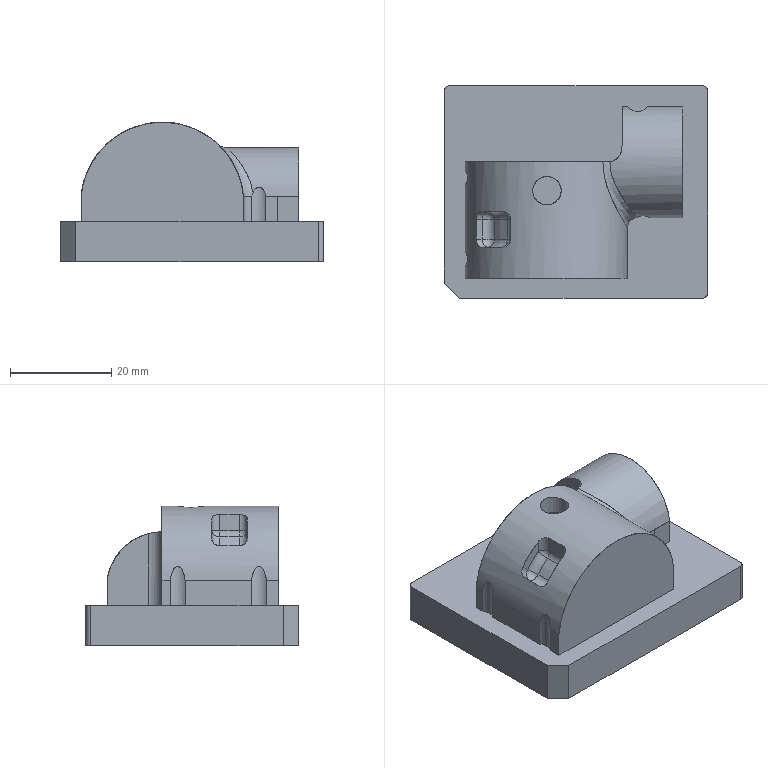NC program | PowerMill | posted with a generic post | part box 52 x 42 x 27.622 mm
Lines 31074 to 31904 of 214543:
N31171 M6
N31172 S18000 M03
N31173 G00 G90 X0.0 Y0.0
N31174 G43 Z9.8022 H28
N31175
N31176 G05 P10000 R4
N31177 X-5.3782 Y0.3338
N31178 Z0.6661
N31179 G01 Z-0.5339 F2400.0
N31180 X-5.0522 Y0.4141 Z-0.5398
N31181 X-4.5942 Z-0.5478
N31182 X-4.1495 Y0.3045 Z-0.5558
N31183 X-3.8382 Y0.1411 Z-0.5619
N31184 X-3.8434 Y0.0036 Z-0.5643
N31185 X-3.9122 Y-0.335 Z-0.5704
N31186 X-4.0514 Y-0.6732 Z-0.5767
N31187 X-4.3199 Y-1.0601 Z-0.585
N31188 X-4.6246 Y-1.3218 Z-0.592
N31189 X-4.8383 Y-1.4461 Z-0.5963
N31190 X-4.9933 Y-1.5363 Z-0.5994
N31191 X-4.997 Y-1.5384 Z-0.5995
N31192 X-5.3352 Y-1.6444 Z-0.6057
N31193 X-5.6736 Y-1.6847 Z-0.6116
N31194 X-6.012 Y-1.6647 Z-0.6175
N31195 X-6.35 Y-1.583 Z-0.6236
N31196 X-6.715 Y-1.4042 Z-0.6307
N31197 X-6.668 Y-1.0173 Z-0.6375
N31198 X-6.5056 Y-0.5891 Z-0.6455
N31199 X-6.2454 Y-0.2121 Z-0.6535
N31200 X-5.9025 Y0.0916 Z-0.6615
N31201 X-5.497 Y0.3045 Z-0.6695
N31202 X-5.0522 Y0.4141 Z-0.6775
N31203 X-4.5942 Z-0.6855
N31204 X-4.1495 Y0.3045 Z-0.6934
N31205 X-3.8382 Y0.1411 Z-0.6996
N31206 X-3.8434 Y0.0036 Z-0.702
N31207 X-3.9122 Y-0.335 Z-0.708
N31208 X-4.0514 Y-0.6732 Z-0.7144
N31209 X-4.3199 Y-1.0601 Z-0.7226
N31210 X-4.6246 Y-1.3218 Z-0.7296
N31211 X-4.8383 Y-1.4461 Z-0.7339
N31212 X-4.8232 Y-1.472
N31213 X-5.305 Y-0.5688 F4000.0
N31214 G03 X-4.8696 Y0.1569 I-0.387 J0.7257
N31215 G03 X-6.5143 I-0.8224 J0.0
N31216 G03 X-5.305 Y-0.5688 I0.8223 J0.0
N31217 G01 X-4.8232 Y-1.472
N31218 X-4.6072 Y-1.3463
N31219 X-4.2975 Y-1.0804
N31220 X-4.0249 Y-0.6876
N31221 X-3.8833 Y-0.3438
N31222 X-3.8136 Y0.0
N31223 X-3.8005 Y0.3438
N31224 X-3.859 Y0.6876
N31225 X-3.9537 Y0.9709
N31226 X-4.1319 Y1.2835
N31227 X-4.284 Y1.4942
N31228 X-4.2975 Y1.5102
N31229 X-4.6413 Y1.8089
N31230 X-4.9851 Y1.9994
N31231 X-5.3289 Y2.1071
N31232 X-5.6727 Y2.1481
N31233 X-6.0165 Y2.1279
N31234 X-6.3004 Y2.0628
N31235 X-6.7041 Y1.8894
N31236 X-6.7094 Y1.8857
N31237 X-6.9842 Y1.6864
N31238 X-7.2966 Y1.3752
N31239 X-7.5019 Y1.0314
N31240 X-7.623 Y0.6876
N31241 X-7.6792 Y0.3438
N31242 X-7.6692 Y0.0
N31243 X-7.5991 Y-0.3438
N31244 X-7.4593 Y-0.6876
N31245 X-7.2269 Y-1.0314
N31246 X-6.8424 Y-1.3752
N31247 X-6.3603 Y-1.6114
N31248 X-6.0165 Y-1.6945
N31249 X-5.6727 Y-1.7148
N31250 X-5.3289 Y-1.6738
N31251 X-4.9851 Y-1.5661
N31252 X-4.9785 Y-1.5624
N31253 X-4.8232 Y-1.472
N31254 X-5.6684 Y0.541 Z-0.6329
N31255 X-5.6503 Y0.6898 Z-0.6355 F2400.0
N31256 X-5.4879 Y1.118 Z-0.6435
N31257 X-5.2277 Y1.495 Z-0.6515
N31258 X-4.8848 Y1.7987 Z-0.6595
N31259 X-4.7821 Y1.8526 Z-0.6615
N31260 X-4.6586 Y1.7842 Z-0.664
N31261 X-4.3189 Y1.4879 Z-0.6719
N31262 X-4.3018 Y1.4676 Z-0.6723
N31263 X-4.1592 Y1.2702 Z-0.6766
N31264 X-3.9812 Y0.957 Z-0.6829
N31265 X-3.8882 Y0.6803 Z-0.688
N31266 X-3.8317 Y0.3418 Z-0.694
N31267 X-3.8355 Y0.2361 Z-0.6958
N31268 X-3.8438 Y0.0035 Z-0.6999
N31269 X-3.9125 Y-0.335 Z-0.7059
N31270 X-4.0522 Y-0.6732 Z-0.7123
N31271 X-4.32 Y-1.06 Z-0.7205
N31272 X-4.6249 Y-1.322 Z-0.7275
N31273 X-4.7541 Y-1.3972 Z-0.7301
N31274 X-4.8848 Y-1.3286 Z-0.7327
N31275 X-5.2277 Y-1.0249 Z-0.7407
N31276 X-5.4879 Y-0.6479 Z-0.7487
N31277 X-5.6503 Y-0.2196 Z-0.7567
N31278 X-5.7055 Y0.2351 Z-0.7647
N31279 X-5.6503 Y0.6898 Z-0.7727
N31280 X-5.4879 Y1.118 Z-0.7807
N31281 X-5.2277 Y1.495 Z-0.7887
N31282 X-4.8848 Y1.7987 Z-0.7966
N31283 X-4.7821 Y1.8526 Z-0.7987
N31284 X-4.6586 Y1.7842 Z-0.8011
N31285 X-4.3189 Y1.4879 Z-0.809
N31286 X-4.3018 Y1.4676 Z-0.8095
N31287 X-4.1592 Y1.2702 Z-0.8137
N31288 X-3.9812 Y0.957 Z-0.82
N31289 X-3.8882 Y0.6803 Z-0.8251
N31290 X-3.8317 Y0.3418 Z-0.8311
N31291 X-3.8355 Y0.2361 Z-0.8329
N31292 X-3.8055 Y0.2351
N31293 X-4.8263 F4000.0
N31294 G03 X-6.4843 I-0.829 J0.0
N31295 G03 X-4.8263 I0.829 J0.0
N31296 G01 X-3.8055
N31297 X-3.8016 Y0.3438
N31298 X-3.859 Y0.6876
N31299 X-3.9537 Y0.9693
N31300 X-4.134 Y1.2865
N31301 X-4.2781 Y1.4861
N31302 X-4.2975 Y1.509
N31303 X-4.6413 Y1.8089
N31304 X-4.9851 Y1.9994
N31305 X-5.3289 Y2.1071
N31306 X-5.6727 Y2.1481
N31307 X-6.0165 Y2.1279
N31308 X-6.3003 Y2.0628
N31309 X-6.7041 Y1.8894
N31310 X-6.7112 Y1.8844
N31311 X-6.9835 Y1.687
N31312 X-7.2953 Y1.3752
N31313 X-7.5006 Y1.0314
N31314 X-7.6218 Y0.6876
N31315 X-7.677 Y0.3438
N31316 X-7.6686 Y0.0
N31317 X-7.5986 Y-0.3438
N31318 X-7.4585 Y-0.6876
N31319 X-7.2258 Y-1.0314
N31320 X-6.8424 Y-1.3752
N31321 X-6.3603 Y-1.6114
N31322 X-6.0165 Y-1.6945
N31323 X-5.6727 Y-1.7148
N31324 X-5.3289 Y-1.6738
N31325 X-4.9851 Y-1.5661
N31326 X-4.9763 Y-1.5612
N31327 X-4.6074 Y-1.3465
N31328 X-4.2975 Y-1.0803
N31329 X-4.0257 Y-0.6876
N31330 X-3.8837 Y-0.3438
N31331 X-3.8139 Y0.0
N31332 X-3.8055 Y0.2351
N31333 X-6.0811 Y0.105 Z-0.7319
N31334 X-6.4496 Y0.0142 Z-0.7385 F2400.0
N31335 X-6.9076 Z-0.7465
N31336 X-7.3523 Y0.1238 Z-0.7545
N31337 X-7.644 Y0.2768 Z-0.7603
N31338 X-7.6454 Y0.3418 Z-0.7614
N31339 X-7.5917 Y0.6802 Z-0.7674
N31340 X-7.472 Y1.0186 Z-0.7737
N31341 X-7.2701 Y1.3566 Z-0.7805
N31342 X-6.9633 Y1.6646 Z-0.7881
N31343 X-6.6957 Y1.8587 Z-0.7939
N31344 X-6.6895 Y1.863 Z-0.794
N31345 X-6.6667 Y1.8727 Z-0.7944
N31346 X-6.291 Y2.0342 Z-0.8016
N31347 X-6.0122 Y2.0981 Z-0.8066
N31348 X-5.6736 Y2.118 Z-0.8125
N31349 X-5.3352 Y2.0776 Z-0.8184
N31350 X-4.997 Y1.9717 Z-0.8246
N31351 X-4.7842 Y1.8538 Z-0.8289
N31352 X-4.8338 Y1.4456 Z-0.836
N31353 X-4.9962 Y1.0173 Z-0.844
N31354 X-5.2564 Y0.6404 Z-0.852
N31355 X-5.5993 Y0.3366 Z-0.86
N31356 X-6.0048 Y0.1238 Z-0.868
N31357 X-6.4496 Y0.0142 Z-0.876
N31358 X-6.9076 Z-0.884
N31359 X-7.3523 Y0.1238 Z-0.892
N31360 X-7.644 Y0.2768 Z-0.8978
N31361 X-7.6454 Y0.3418 Z-0.8989
N31362 X-7.5917 Y0.6802 Z-0.9049
N31363 X-7.472 Y1.0186 Z-0.9111
N31364 X-7.2701 Y1.3566 Z-0.918
N31365 X-6.9633 Y1.6646 Z-0.9256
N31366 X-6.6957 Y1.8587 Z-0.9314
N31367 X-6.6895 Y1.863 Z-0.9315
N31368 X-6.6667 Y1.8727 Z-0.9319
N31369 X-6.6786 Y1.9003
N31370 X-6.1941 Y0.9919 F4000.0
N31371 G03 X-6.6309 Y0.2639 I0.3883 J-0.728
N31372 G03 X-4.9808 I0.8251 J0.0
N31373 G03 X-6.1941 Y0.9919 I-0.825 J0.0
N31374 G01 X-6.6786 Y1.9003
N31375 X-6.7041 Y1.8893
N31376 X-6.713 Y1.8832
N31377 X-6.9829 Y1.6875
N31378 X-7.294 Y1.3752
N31379 X-7.4993 Y1.0314
N31380 X-7.6209 Y0.6876
N31381 X-7.6754 Y0.3438
N31382 X-7.668 Y0.0
N31383 X-7.5981 Y-0.3438
N31384 X-7.4577 Y-0.6876
N31385 X-7.2247 Y-1.0314
N31386 X-6.8424 Y-1.3752
N31387 X-6.3603 Y-1.6114
N31388 X-6.0165 Y-1.6945
N31389 X-5.6727 Y-1.7148
N31390 X-5.3289 Y-1.6738
N31391 X-4.9851 Y-1.5661
N31392 X-4.9741 Y-1.56
N31393 X-4.6077 Y-1.3467
N31394 X-4.2975 Y-1.0802
N31395 X-4.0265 Y-0.6876
N31396 X-3.8845 Y-0.3438
N31397 X-3.8142 Y0.0
N31398 X-3.8028 Y0.3438
N31399 X-3.8591 Y0.6876
N31400 X-3.9537 Y0.968
N31401 X-4.136 Y1.2893
N31402 X-4.2727 Y1.4786
N31403 X-4.2975 Y1.5078
N31404 X-4.6413 Y1.8089
N31405 X-4.9851 Y1.9994
N31406 X-5.3289 Y2.1071
N31407 X-5.6727 Y2.1481
N31408 X-6.0165 Y2.1279
N31409 X-6.3003 Y2.0628
N31410 X-6.6786 Y1.9003
N31411 X-6.0784 Y0.1056 Z-0.8309
N31412 X-6.4497 Y0.0141 Z-0.8376 F2400.0
N31413 X-6.9078 Z-0.8456
N31414 X-7.3525 Y0.1237 Z-0.8536
N31415 X-7.6431 Y0.2762 Z-0.8593
N31416 X-7.6444 Y0.3417 Z-0.8604
N31417 X-7.5908 Y0.6802 Z-0.8664
N31418 X-7.4707 Y1.0186 Z-0.8727
N31419 X-7.2688 Y1.3567 Z-0.8796
N31420 X-6.9627 Y1.6652 Z-0.8871
N31421 X-6.6975 Y1.8575 Z-0.8929
N31422 X-6.6895 Y1.863 Z-0.893
N31423 X-6.6669 Y1.8727 Z-0.8935
N31424 X-6.291 Y2.0342 Z-0.9006
N31425 X-6.0122 Y2.0981 Z-0.9056
N31426 X-5.6736 Y2.118 Z-0.9115
N31427 X-5.3352 Y2.0776 Z-0.9175
N31428 X-4.997 Y1.9717 Z-0.9236
N31429 X-4.7844 Y1.8539 Z-0.9279
N31430 X-4.834 Y1.4455 Z-0.9351
N31431 X-4.9964 Y1.0173 Z-0.9431
N31432 X-5.2566 Y0.6403 Z-0.9511
N31433 X-5.5994 Y0.3366 Z-0.959
N31434 X-6.005 Y0.1237 Z-0.967
N31435 X-6.4497 Y0.0141 Z-0.975
N31436 X-6.9078 Z-0.983
N31437 X-7.3525 Y0.1237 Z-0.991
N31438 X-7.6431 Y0.2762 Z-0.9967
N31439 X-7.6444 Y0.3417 Z-0.9979
N31440 X-7.5908 Y0.6802 Z-1.0039
N31441 X-7.4707 Y1.0186 Z-1.0101
N31442 X-7.2688 Y1.3567 Z-1.017
N31443 X-6.9627 Y1.6652 Z-1.0246
N31444 X-6.6975 Y1.8575 Z-1.0303
N31445 X-6.6895 Y1.863 Z-1.0305
N31446 X-6.6669 Y1.8727 Z-1.0309
N31447 X-6.6788 Y1.9002
N31448 X-6.1943 Y0.9919 F4000.0
N31449 G03 X-6.631 Y0.264 I0.3882 J-0.7279
N31450 G03 X-4.9811 I0.8249 J0.0
N31451 G03 X-6.1943 Y0.9919 I-0.825 J0.0
N31452 G01 X-6.6788 Y1.9002
N31453 X-6.7041 Y1.8893
N31454 X-6.7148 Y1.882
N31455 X-6.9822 Y1.688
N31456 X-7.2927 Y1.3752
N31457 X-7.498 Y1.0314
N31458 X-7.62 Y0.6876
N31459 X-7.6745 Y0.3438
N31460 X-7.6674 Y0.0
N31461 X-7.5975 Y-0.3438
N31462 X-7.4568 Y-0.6876
N31463 X-7.2236 Y-1.0314
N31464 X-6.8424 Y-1.3752
N31465 X-6.3603 Y-1.6114
N31466 X-6.0165 Y-1.6945
N31467 X-5.6727 Y-1.7148
N31468 X-5.3289 Y-1.6738
N31469 X-4.9851 Y-1.5661
N31470 X-4.9719 Y-1.5587
N31471 X-4.6079 Y-1.3469
N31472 X-4.2975 Y-1.0801
N31473 X-4.0274 Y-0.6876
N31474 X-3.8853 Y-0.3438
N31475 X-3.8145 Y0.0
N31476 X-3.804 Y0.3438
N31477 X-3.8591 Y0.6876
N31478 X-3.9537 Y0.9673
N31479 X-4.1375 Y1.2916
N31480 X-4.2676 Y1.4717
N31481 X-4.2975 Y1.5066
N31482 X-4.6413 Y1.8089
N31483 X-4.9851 Y1.9994
N31484 X-5.3289 Y2.1071
N31485 X-5.6727 Y2.1481
N31486 X-6.0165 Y2.1279
N31487 X-6.3003 Y2.0628
N31488 X-6.6788 Y1.9002
N31489 X-6.0684 Y0.0395 Z-0.9299
N31490 X-6.2959 Y-0.0799 Z-0.9344 F2400.0
N31491 X-6.7406 Y-0.1895 Z-0.9424
N31492 X-7.1987 Z-0.9504
N31493 X-7.6187 Y-0.086 Z-0.9579
N31494 X-7.6369 Y0.0033 Z-0.9595
N31495 X-7.6434 Y0.3417 Z-0.9654
N31496 X-7.5899 Y0.6802 Z-0.9714
N31497 X-7.4691 Y1.0195 Z-0.9777
N31498 X-7.4626 Y1.0323 Z-0.9779
N31499 X-7.3113 Y1.2857 Z-0.9831
N31500 X-7.1364 Y1.4902 Z-0.9878
N31501 X-6.9649 Y1.663 Z-0.992
N31502 X-6.952 Y1.6724 Z-0.9923
N31503 X-6.6892 Y1.8631 Z-0.998
N31504 X-6.291 Y2.0342 Z-1.0055
N31505 X-6.0122 Y2.098 Z-1.0105
N31506 X-5.6736 Y2.118 Z-1.0164
N31507 X-5.3352 Y2.0776 Z-1.0224
N31508 X-5.1072 Y2.0062 Z-1.0266
N31509 X-5.0696 Y1.6966 Z-1.032
N31510 X-5.1248 Y1.2419 Z-1.04
N31511 X-5.2873 Y0.8137 Z-1.048
N31512 X-5.5475 Y0.4367 Z-1.056
N31513 X-5.8903 Y0.133 Z-1.064
N31514 X-6.2959 Y-0.0799 Z-1.072
N31515 X-6.7406 Y-0.1895 Z-1.08
N31516 X-7.1987 Z-1.088
N31517 X-7.6187 Y-0.086 Z-1.0955
N31518 X-7.6369 Y0.0033 Z-1.0971
N31519 X-7.6434 Y0.3417 Z-1.103
N31520 X-7.5899 Y0.6802 Z-1.109
N31521 X-7.4691 Y1.0195 Z-1.1153
N31522 X-7.4626 Y1.0323 Z-1.1155
N31523 X-7.3113 Y1.2857 Z-1.1207
N31524 X-7.1364 Y1.4902 Z-1.1254
N31525 X-6.9649 Y1.663 Z-1.1296
N31526 X-6.952 Y1.6724 Z-1.1299
N31527 X-6.9696 Y1.6966
N31528 X-6.216 Y0.7888 F4000.0
N31529 G03 X-6.3192 Y-0.2477 I0.4737 J-0.5706
N31530 G01 X-6.3174 Y-0.2499
N31531 G03 X-5.2667 Y-0.3546 I0.5769 J0.4659
N31532 G03 X-5.1763 Y0.6974 I-0.4738 J0.5706
N31533 G01 X-5.1781 Y0.6996
N31534 G03 X-6.216 Y0.7888 I-0.5642 J-0.4814
N31535 G01 X-6.9696 Y1.6966
N31536 X-6.9844 Y1.6859
N31537 X-7.1585 Y1.5105
N31538 X-7.3357 Y1.3032
N31539 X-7.4889 Y1.0468
N31540 X-7.4967 Y1.0314
N31541 X-7.6191 Y0.6876
N31542 X-7.6735 Y0.3438
N31543 X-7.6668 Y0.0
N31544 X-7.597 Y-0.3438
N31545 X-7.456 Y-0.6876
N31546 X-7.2225 Y-1.0314
N31547 X-6.8424 Y-1.3752
N31548 X-6.3603 Y-1.6114
N31549 X-6.0165 Y-1.6945
N31550 X-5.6727 Y-1.7148
N31551 X-5.3289 Y-1.6738
N31552 X-4.9851 Y-1.5661
N31553 X-4.9762 Y-1.5611
N31554 X-4.9697 Y-1.5575
N31555 X-4.6081 Y-1.3471
N31556 X-4.2975 Y-1.08
N31557 X-4.0282 Y-0.6876
N31558 X-3.8861 Y-0.3438
N31559 X-3.8148 Y0.0
N31560 X-3.8051 Y0.3438
N31561 X-3.8591 Y0.6876
N31562 X-3.9537 Y0.9673
N31563 X-4.1388 Y1.2934
N31564 X-4.2629 Y1.4653
N31565 X-4.2975 Y1.5054
N31566 X-4.6413 Y1.8089
N31567 X-4.9851 Y1.9994
N31568 X-5.3289 Y2.1071
N31569 X-5.6727 Y2.1481
N31570 X-6.0165 Y2.1278
N31571 X-6.3003 Y2.0628
N31572 X-6.7041 Y1.8893
N31573 X-6.9696 Y1.6966
N31574 X-5.4401 Y-0.0263 Z-1.0289
N31575 X-5.2402 Y-0.2035 Z-1.0335 F2400.0
N31576 X-4.98 Y-0.5804 Z-1.0415
N31577 X-4.8175 Y-1.0087 Z-1.0495
N31578 X-4.7693 Y-1.4062 Z-1.0565
N31579 X-4.9823 Y-1.5302 Z-1.0608
N31580 X-4.9907 Y-1.5349 Z-1.061
N31581 X-4.997 Y-1.5383 Z-1.0611
N31582 X-5.3352 Y-1.6444 Z-1.0673
N31583 X-5.6736 Y-1.6847 Z-1.0732
N31584 X-6.012 Y-1.6647 Z-1.0792
N31585 X-6.35 Y-1.583 Z-1.0852
N31586 X-6.6491 Y-1.4365 Z-1.091
N31587 X-6.8254 Y-1.3501 Z-1.0945
N31588 X-7.1986 Y-1.0116 Z-1.1033
N31589 X-7.4286 Y-0.6733 Z-1.1104
N31590 X-7.5676 Y-0.335 Z-1.1168
N31591 X-7.6362 Y0.0033 Z-1.1228
N31592 X-7.639 Y0.1541 Z-1.1254
N31593 X-7.3361 Y0.3131 Z-1.1314
N31594 X-6.8914 Y0.4227 Z-1.1394
N31595 X-6.4333 Z-1.1474
N31596 X-5.9886 Y0.3131 Z-1.1554
N31597 X-5.583 Y0.1003 Z-1.1634
N31598 X-5.2402 Y-0.2035 Z-1.1714
N31599 X-4.98 Y-0.5804 Z-1.1794
N31600 X-4.8175 Y-1.0087 Z-1.1874
N31601 X-4.7693 Y-1.4062 Z-1.1944
N31602 X-4.9823 Y-1.5302 Z-1.1987
N31603 X-4.9907 Y-1.5349 Z-1.1988
N31604 X-4.997 Y-1.5383 Z-1.1989
N31605 X-5.3352 Y-1.6444 Z-1.2051
N31606 X-5.6736 Y-1.6847 Z-1.2111
N31607 X-6.012 Y-1.6647 Z-1.217
N31608 X-6.35 Y-1.583 Z-1.2231
N31609 X-6.6491 Y-1.4365 Z-1.2289
N31610 X-6.6623 Y-1.4634
N31611 X-6.1908 Y-0.5793 F4000.0
N31612 G03 X-4.9682 Y0.1543 I0.3912 J0.7336
N31613 G03 X-6.631 I-0.8314 J0.0
N31614 G03 X-6.1908 Y-0.5793 I0.8314 J0.0
N31615 G01 X-6.6623 Y-1.4634
N31616 X-6.3603 Y-1.6114
N31617 X-6.0165 Y-1.6945
N31618 X-5.6727 Y-1.7148
N31619 X-5.3289 Y-1.6738
N31620 X-4.9851 Y-1.5661
N31621 X-4.9762 Y-1.5611
N31622 X-4.9675 Y-1.5563
N31623 X-4.6085 Y-1.3474
N31624 X-4.2975 Y-1.0795
N31625 X-4.0291 Y-0.6876
N31626 X-3.8869 Y-0.3438
N31627 X-3.8151 Y0.0
N31628 X-3.8061 Y0.3438
N31629 X-3.8592 Y0.6876
N31630 X-3.9537 Y0.9672
N31631 X-4.14 Y1.2952
N31632 X-4.257 Y1.4571
N31633 X-4.2975 Y1.5036
N31634 X-4.6413 Y1.8089
N31635 X-4.9851 Y1.9994
N31636 X-5.3289 Y2.1071
N31637 X-5.6727 Y2.1481
N31638 X-6.0165 Y2.1278
N31639 X-6.3003 Y2.0628
N31640 X-6.7041 Y1.8893
N31641 X-6.9847 Y1.6857
N31642 X-7.1578 Y1.5113
N31643 X-7.3361 Y1.3027
N31644 X-7.4813 Y1.0596
N31645 X-7.4955 Y1.0314
N31646 X-7.618 Y0.6876
N31647 X-7.6725 Y0.3438
N31648 X-7.6662 Y0.0
N31649 X-7.5965 Y-0.3438
N31650 X-7.4552 Y-0.6876
N31651 X-7.2214 Y-1.0314
N31652 X-6.8424 Y-1.3752
N31653 X-6.6623 Y-1.4634
N31654 X-5.3878 Y0.3304 Z-1.1279
N31655 X-5.0543 Y0.4126 Z-1.1339 F2400.0
N31656 X-4.5962 Z-1.1419
N31657 X-4.1515 Y0.3029 Z-1.1499
N31658 X-3.8418 Y0.1404 Z-1.156
N31659 X-3.8453 Y0.0035 Z-1.1583
N31660 X-3.9166 Y-0.3349 Z-1.1644
N31661 X-4.0565 Y-0.6732 Z-1.1708
N31662 X-4.32 Y-1.0588 Z-1.1789
N31663 X-4.6264 Y-1.3232 Z-1.186
N31664 X-4.8403 Y-1.4477 Z-1.1903
N31665 X-4.9801 Y-1.529 Z-1.1931
N31666 X-4.997 Y-1.5383 Z-1.1935
N31667 X-5.3352 Y-1.6444 Z-1.1996
N31668 X-5.6736 Y-1.6847 Z-1.2056
N31669 X-6.012 Y-1.6647 Z-1.2115
N31670 X-6.35 Y-1.583 Z-1.2176
N31671 X-6.7167 Y-1.4033 Z-1.2247
N31672 X-6.67 Y-1.0189 Z-1.2315
N31673 X-6.5076 Y-0.5906 Z-1.2395
N31674 X-6.2474 Y-0.2136 Z-1.2475
N31675 X-5.9046 Y0.0901 Z-1.2554
N31676 X-5.499 Y0.3029 Z-1.2634
N31677 X-5.0543 Y0.4126 Z-1.2714
N31678 X-4.5962 Z-1.2794
N31679 X-4.1515 Y0.3029 Z-1.2874
N31680 X-3.8418 Y0.1404 Z-1.2935
N31681 X-3.8453 Y0.0035 Z-1.2959
N31682 X-3.9166 Y-0.3349 Z-1.3019
N31683 X-4.0565 Y-0.6732 Z-1.3083
N31684 X-4.32 Y-1.0588 Z-1.3165
N31685 X-4.6264 Y-1.3232 Z-1.3236
N31686 X-4.8403 Y-1.4477 Z-1.3279
N31687 X-4.8253 Y-1.4736
N31688 X-5.3041 Y-0.5758 F4000.0
N31689 G03 X-4.8676 Y0.1517 I-0.388 J0.7275
N31690 G03 X-6.5166 I-0.8245 J0.0
N31691 G03 X-5.3041 Y-0.5758 I0.8245 J0.0
N31692 G01 X-4.8253 Y-1.4736
N31693 X-4.6089 Y-1.3477
N31694 X-4.2975 Y-1.0789
N31695 X-4.0299 Y-0.6876
N31696 X-3.8879 Y-0.3438
N31697 X-3.8154 Y0.0
N31698 X-3.8066 Y0.3438
N31699 X-3.8592 Y0.6876
N31700 X-3.9537 Y0.9672
N31701 X-4.1412 Y1.297
N31702 X-4.2241 Y1.4117
N31703 X-4.6413 Y1.8089
N31704 X-4.9851 Y1.9994
N31705 X-5.3289 Y2.1071
N31706 X-5.6727 Y2.1481
N31707 X-6.0165 Y2.1278
N31708 X-6.3003 Y2.0628
N31709 X-6.7041 Y1.8893
N31710 X-6.985 Y1.6855
N31711 X-7.1572 Y1.512
N31712 X-7.3365 Y1.3022
N31713 X-7.4758 Y1.0688
N31714 X-7.4945 Y1.0314
N31715 X-7.6167 Y0.6876
N31716 X-7.6715 Y0.3438
N31717 X-7.6651 Y0.0
N31718 X-7.596 Y-0.3438
N31719 X-7.4544 Y-0.6876
N31720 X-7.2203 Y-1.0314
N31721 X-6.8424 Y-1.3752
N31722 X-6.3603 Y-1.6114
N31723 X-6.0165 Y-1.6945
N31724 X-5.6727 Y-1.7148
N31725 X-5.3289 Y-1.6738
N31726 X-4.9851 Y-1.5661
N31727 X-4.9653 Y-1.5551
N31728 X-4.8253 Y-1.4736
N31729 X-5.3894 Y0.33 Z-1.2269
N31730 X-5.054 Y0.4127 Z-1.2329 F2400.0
N31731 X-4.5959 Z-1.2409
N31732 X-4.1512 Y0.3031 Z-1.2489
N31733 X-3.8422 Y0.1409 Z-1.255
N31734 X-3.8457 Y0.0035 Z-1.2574
N31735 X-3.9175 Y-0.3349 Z-1.2634
N31736 X-4.0573 Y-0.6733 Z-1.2698
N31737 X-4.3201 Y-1.0582 Z-1.2779
N31738 X-4.6269 Y-1.3235 Z-1.285
N31739 X-4.8401 Y-1.4475 Z-1.2893
N31740 X-4.9779 Y-1.5278 Z-1.2921
N31741 X-4.997 Y-1.5383 Z-1.2925
N31742 X-5.3352 Y-1.6443 Z-1.2987
N31743 X-5.6736 Y-1.6847 Z-1.3046
N31744 X-6.012 Y-1.6647 Z-1.3105
N31745 X-6.35 Y-1.583 Z-1.3166
N31746 X-6.7165 Y-1.4035 Z-1.3237
N31747 X-6.6698 Y-1.0188 Z-1.3305
N31748 X-6.5073 Y-0.5905 Z-1.3385
N31749 X-6.2471 Y-0.2135 Z-1.3465
N31750 X-5.9043 Y0.0902 Z-1.3545
N31751 X-5.4987 Y0.3031 Z-1.3624
N31752 X-5.054 Y0.4127 Z-1.3704
N31753 X-4.5959 Z-1.3784
N31754 X-4.1512 Y0.3031 Z-1.3864
N31755 X-3.8422 Y0.1409 Z-1.3925
N31756 X-3.8457 Y0.0035 Z-1.3949
N31757 X-3.9175 Y-0.3349 Z-1.401
N31758 X-4.0573 Y-0.6733 Z-1.4073
N31759 X-4.3201 Y-1.0582 Z-1.4155
N31760 X-4.6269 Y-1.3235 Z-1.4226
N31761 X-4.8401 Y-1.4475 Z-1.4269
N31762 X-4.825 Y-1.4735
N31763 X-5.3042 Y-0.5749 F4000.0
N31764 G03 X-4.8679 Y0.1521 I-0.3877 J0.727
N31765 G03 X-6.5159 I-0.824 J0.0
N31766 G03 X-5.3042 Y-0.5749 I0.824 J0.0
N31767 G01 X-4.825 Y-1.4735
N31768 X-4.6094 Y-1.348
N31769 X-4.2975 Y-1.0783
N31770 X-4.0308 Y-0.6876
N31771 X-3.8888 Y-0.3438
N31772 X-3.8157 Y0.0
N31773 X-3.8071 Y0.3438
N31774 X-3.8593 Y0.6876
N31775 X-3.9537 Y0.9672
N31776 X-4.1425 Y1.2988
N31777 X-4.2234 Y1.4108
N31778 X-4.6413 Y1.8089
N31779 X-4.9851 Y1.9994
N31780 X-5.3289 Y2.1071
N31781 X-5.6727 Y2.1481
N31782 X-6.0165 Y2.1278
N31783 X-6.3003 Y2.0628
N31784 X-6.7041 Y1.8893
N31785 X-6.9852 Y1.6853
N31786 X-7.1565 Y1.5127
N31787 X-7.3368 Y1.3017
N31788 X-7.4721 Y1.0751
N31789 X-7.4938 Y1.0314
N31790 X-7.6159 Y0.6876
N31791 X-7.6706 Y0.3438
N31792 X-7.6641 Y0.0
N31793 X-7.5955 Y-0.3438
N31794 X-7.4536 Y-0.6876
N31795 X-7.2192 Y-1.0314
N31796 X-6.8424 Y-1.3752
N31797 X-6.3603 Y-1.6114
N31798 X-6.0165 Y-1.6945
N31799 X-5.6727 Y-1.7148
N31800 X-5.3289 Y-1.6738
N31801 X-4.9851 Y-1.5661
N31802 X-4.9631 Y-1.5539
N31803 X-4.825 Y-1.4735
N31804 X-6.0144 Y-0.0306 Z-1.3258
N31805 X-6.2011 Y-0.1961 Z-1.3302 F2400.0
N31806 X-6.6067 Y-0.4089 Z-1.3382
N31807 X-7.0514 Y-0.5186 Z-1.3462
N31808 X-7.49 Z-1.3538
N31809 X-7.5655 Y-0.3351 Z-1.3573
N31810 X-7.6331 Y0.0033 Z-1.3633
N31811 X-7.6396 Y0.3417 Z-1.3692
N31812 X-7.586 Y0.6802 Z-1.3752
N31813 X-7.4657 Y1.0197 Z-1.3815
N31814 X-7.4434 Y1.0648 Z-1.3824
N31815 X-7.3127 Y1.2836 Z-1.3868
N31816 X-7.2577 Y1.3481 Z-1.3883
N31817 X-7.1338 Y1.4931 Z-1.3916
N31818 X-6.9659 Y1.6623 Z-1.3958
N31819 X-6.6892 Y1.8631 Z-1.4018
N31820 X-6.291 Y2.0342 Z-1.4093
N31821 X-6.0122 Y2.098 Z-1.4143
N31822 X-5.6736 Y2.118 Z-1.4202
N31823 X-5.5419 Y2.1022 Z-1.4225
N31824 X-5.4357 Y1.8223 Z-1.4278
N31825 X-5.3805 Y1.3676 Z-1.4358
N31826 X-5.4357 Y0.9129 Z-1.4438
N31827 X-5.5981 Y0.4846 Z-1.4517
N31828 X-5.8583 Y0.1077 Z-1.4597
N31829 X-6.2011 Y-0.1961 Z-1.4677
N31830 X-6.6067 Y-0.4089 Z-1.4757
N31831 X-7.0514 Y-0.5186 Z-1.4837
N31832 X-7.49 Z-1.4914
N31833 X-7.5655 Y-0.3351 Z-1.4948
N31834 X-7.6331 Y0.0033 Z-1.5009
N31835 X-7.6396 Y0.3417 Z-1.5068
N31836 X-7.586 Y0.6802 Z-1.5127
N31837 X-7.4657 Y1.0197 Z-1.519
N31838 X-7.4434 Y1.0648 Z-1.5199
N31839 X-7.3127 Y1.2836 Z-1.5244
N31840 X-7.2577 Y1.3481 Z-1.5258
N31841 X-7.2805 Y1.3676
N31842 X-6.4649 Y0.7559 F4000.0
N31843 G03 X-6.6295 Y0.2622 I0.6583 J-0.4937
N31844 G03 X-4.9836 I0.8229 J0.0
N31845 G03 X-6.4649 Y0.7559 I-0.823 J0.0
N31846 G01 X-7.2805 Y1.3676
N31847 X-7.3372 Y1.3012
N31848 X-7.4698 Y1.0792
N31849 X-7.4933 Y1.0314
N31850 X-7.6152 Y0.6876
N31851 X-7.6696 Y0.3438
N31852 X-7.6631 Y0.0
N31853 X-7.5944 Y-0.3438
N31854 X-7.4528 Y-0.6876
N31855 X-7.2178 Y-1.0314
N31856 X-6.8424 Y-1.3752
N31857 X-6.3603 Y-1.6114
N31858 X-6.0165 Y-1.6945
N31859 X-5.6727 Y-1.7148
N31860 X-5.3289 Y-1.6738
N31861 X-4.9851 Y-1.566
N31862 X-4.9609 Y-1.5526
N31863 X-4.6098 Y-1.3483
N31864 X-4.2975 Y-1.0777
N31865 X-4.0317 Y-0.6876
N31866 X-3.8897 Y-0.3438
N31867 X-3.8164 Y0.0
N31868 X-3.8075 Y0.3438
N31869 X-3.8594 Y0.6876
N31870 X-3.9537 Y0.9672
N31871 X-4.1437 Y1.3006
N31872 X-4.2226 Y1.4099
N31873 X-4.6413 Y1.8089
N31874 X-4.9851 Y1.9994
N31875 X-5.3289 Y2.1071
N31876 X-5.6727 Y2.1481
N31877 X-6.0165 Y2.1278
N31878 X-6.3003 Y2.0628
N31879 X-6.7041 Y1.8893
N31880 X-6.9855 Y1.6851
N31881 X-7.1559 Y1.5134
N31882 X-7.2805 Y1.3676
N31883 X-5.8902 Y0.5217 Z-1.4248
N31884 X-6.0404 Y0.9179 Z-1.4322 F2400.0
N31885 X-6.0957 Y1.3726 Z-1.4402
N31886 X-6.0404 Y1.8273 Z-1.4482
N31887 X-5.9361 Y2.1025 Z-1.4533
N31888 X-5.6736 Y2.1179 Z-1.4579
N31889 X-5.3352 Y2.0776 Z-1.4639
N31890 X-4.997 Y1.9717 Z-1.4701
N31891 X-4.6592 Y1.7845 Z-1.4768
N31892 X-4.2446 Y1.3891 Z-1.4868
N31893 X-4.22 Y1.355 Z-1.4875
N31894 X-4.1703 Y1.2862 Z-1.489
N31895 X-3.9812 Y0.9549 Z-1.4957
N31896 X-3.8891 Y0.6805 Z-1.5007
N31897 X-3.8381 Y0.342 Z-1.5067
N31898 X-3.8473 Y0.0042 Z-1.5126
N31899 X-3.961 Y-0.4379 Z-1.5206
N31900 X-3.9922 Y-0.5136 Z-1.522
N31901 X-4.4247 Z-1.5295
N31902 X-4.8694 Y-0.4039 Z-1.5375
N31903 X-5.275 Y-0.1911 Z-1.5455
N31904 X-5.6178 Y0.1127 Z-1.5535
N31905 X-5.878 Y0.4896 Z-1.5615
N31906 X-6.0404 Y0.9179 Z-1.5695
N31907 X-6.0957 Y1.3726 Z-1.5775
N31908 X-6.0404 Y1.8273 Z-1.5855
N31909 X-5.9361 Y2.1025 Z-1.5906
N31910 X-5.6736 Y2.1179 Z-1.5952
N31911 X-5.3352 Y2.0776 Z-1.6012
N31912 X-4.997 Y1.9717 Z-1.6074
N31913 X-4.6592 Y1.7845 Z-1.6141
N31914 X-4.2446 Y1.3891 Z-1.6241
N31915 X-4.22 Y1.355 Z-1.6248
N31916 X-4.1957 Y1.3726
N31917 X-5.0155 Y0.7577 F4000.0
N31918 G03 X-6.4979 Y0.2636 I-0.6588 J-0.4941
N31919 G03 X-4.8508 I0.8236 J0.0
N31920 G03 X-5.0155 Y0.7577 I-0.8235 J0.0
N31921 G01 X-4.1957 Y1.3726
N31922 X-4.2219 Y1.4089
N31923 X-4.6413 Y1.8089
N31924 X-4.9851 Y1.9994
N31925 X-5.3289 Y2.1071
N31926 X-5.6727 Y2.1481
N31927 X-6.0165 Y2.1278
N31928 X-6.3003 Y2.0628
N31929 X-6.7041 Y1.8893
N31930 X-6.9857 Y1.6849
N31931 X-7.1552 Y1.5142
N31932 X-7.3376 Y1.3007
N31933 X-7.4691 Y1.0804
N31934 X-7.4933 Y1.0314
N31935 X-7.6146 Y0.6876
N31936 X-7.6687 Y0.3438
N31937 X-7.662 Y0.0
N31938 X-7.5931 Y-0.3438
N31939 X-7.452 Y-0.6876
N31940 X-7.2163 Y-1.0314
N31941 X-6.8424 Y-1.3752
N31942 X-6.3603 Y-1.6114
N31943 X-6.0165 Y-1.6945
N31944 X-5.6727 Y-1.7148
N31945 X-5.3289 Y-1.6738
N31946 X-4.9851 Y-1.566
N31947 X-4.9587 Y-1.5514
N31948 X-4.6102 Y-1.3486
N31949 X-4.2975 Y-1.077
N31950 X-4.0325 Y-0.6876
N31951 X-4.0273 Y-0.6772
N31952 X-3.9324 Y-0.4474
N31953 X-3.8174 Y0.0
N31954 X-3.808 Y0.3438
N31955 X-3.8598 Y0.6876
N31956 X-3.9537 Y0.9672
N31957 X-4.145 Y1.3024
N31958 X-4.1957 Y1.3726
N31959 X-5.5777 Y-0.0984 Z-1.5238
N31960 X-5.4287 Y-0.4914 Z-1.5312 F2400.0
N31961 X-5.3735 Y-0.9461 Z-1.5391
N31962 X-5.4287 Y-1.4008 Z-1.5471
N31963 X-5.5298 Y-1.6675 Z-1.5521
N31964 X-5.6736 Y-1.6847 Z-1.5546
N31965 X-6.012 Y-1.6647 Z-1.5606
N31966 X-6.35 Y-1.583 Z-1.5666
N31967 X-6.8254 Y-1.3501 Z-1.5759
N31968 X-7.1828 Y-1.0216 Z-1.5843
N31969 X-7.1915 Y-1.0124 Z-1.5846
N31970 X-7.2487 Y-0.9291 Z-1.5863
N31971 X-7.4246 Y-0.6733 Z-1.5917
N31972 X-7.5631 Y-0.3351 Z-1.5981
N31973 X-7.6311 Y0.0033 Z-1.6041
N31974 X-7.6378 Y0.3418 Z-1.6101
N31975 X-7.5852 Y0.6802 Z-1.616
N31976 X-7.4937 Y0.94 Z-1.6208
N31977 X-7.0444 Z-1.6287
N31978 X-6.5997 Y0.8304 Z-1.6367
N31979 X-6.1941 Y0.6176 Z-1.6447
N31980 X-5.8513 Y0.3138 Z-1.6527
N31981 X-5.5911 Y-0.0631 Z-1.6607
N31982 X-5.4287 Y-0.4914 Z-1.6686
N31983 X-5.3735 Y-0.9461 Z-1.6766
N31984 X-5.4287 Y-1.4008 Z-1.6846
N31985 X-5.5298 Y-1.6675 Z-1.6896
N31986 X-5.6736 Y-1.6847 Z-1.6921
N31987 X-6.012 Y-1.6647 Z-1.6981
N31988 X-6.35 Y-1.583 Z-1.7041
N31989 X-6.8254 Y-1.3501 Z-1.7134
N31990 X-7.1828 Y-1.0216 Z-1.7218
N31991 X-7.1915 Y-1.0124 Z-1.7221
N31992 X-7.2487 Y-0.9291 Z-1.7238
N31993 X-7.2735 Y-0.9461
N31994 X-6.4612 Y-0.3369 F4000.0
N31995 G03 X-4.9724 Y0.1594 I0.6617 J0.4963
N31996 G03 X-6.6266 I-0.8271 J0.0
N31997 G03 X-6.4612 Y-0.3369 I0.8271 J0.0
N31998 G01 X-7.2735 Y-0.9461
N31999 X-7.2148 Y-1.0314
N32000 X-7.2038 Y-1.043
N32001 X-6.8431 Y-1.3746